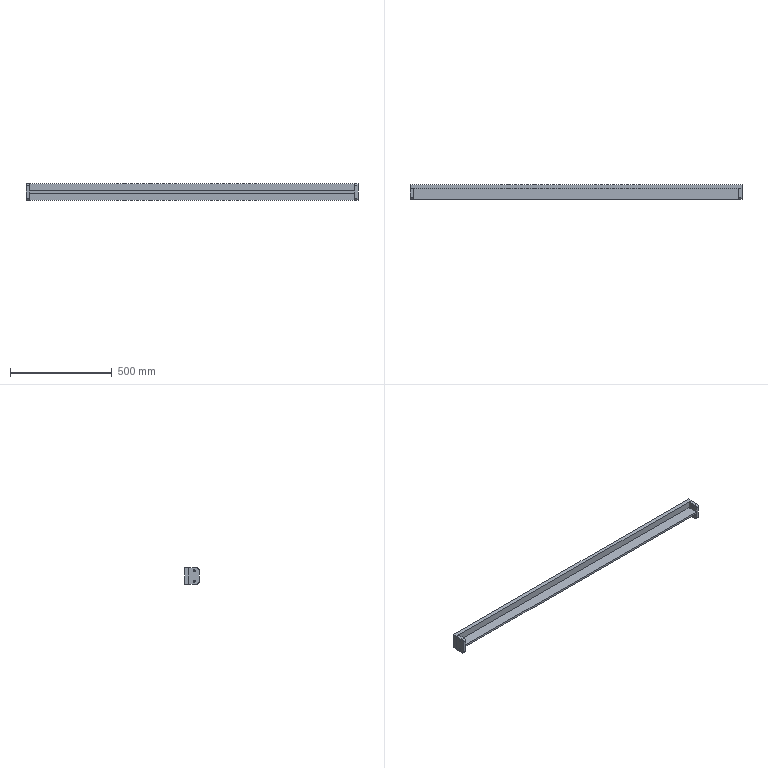Part | SolidWorks | features BaseBody 4 | 4 solids | 36 faces | box 1632 x 70 x 80 mm | volume 3525010 mm3 | plane 24 | cylinder 12 | commonest cylinder face diameters 10.2 x8 20 x4
STEP:
#1=CARTESIAN_POINT('',(-816.,-10.,-40.));
#2=VERTEX_POINT('',#1);
#3=CARTESIAN_POINT('',(-816.,10.,-40.));
#4=VERTEX_POINT('',#3);
#5=CARTESIAN_POINT('',(-816.,10.,-40.));
#6=DIRECTION('',(0.,1.,0.));
#7=VECTOR('',#6,1000.);
#8=LINE('',#5,#7);
#9=EDGE_CURVE('',#2,#4,#8,.T.);
#10=ORIENTED_EDGE('',*,*,#9,.T.);
#11=CARTESIAN_POINT('',(816.,10.,-40.));
#12=VERTEX_POINT('',#11);
#13=CARTESIAN_POINT('',(816.,10.,-40.));
#14=DIRECTION('',(-1.,0.,0.));
#15=VECTOR('',#14,1000.);
#16=LINE('',#13,#15);
#17=EDGE_CURVE('',#12,#4,#16,.T.);
#18=ORIENTED_EDGE('',*,*,#17,.F.);
#19=CARTESIAN_POINT('',(816.,-10.,-40.));
#20=VERTEX_POINT('',#19);
#21=CARTESIAN_POINT('',(816.,10.,-40.));
#22=DIRECTION('',(0.,1.,0.));
#23=VECTOR('',#22,1000.);
#24=LINE('',#21,#23);
#25=EDGE_CURVE('',#20,#12,#24,.T.);
#26=ORIENTED_EDGE('',*,*,#25,.F.);
#27=CARTESIAN_POINT('',(816.,-10.,-40.));
#28=DIRECTION('',(-1.,0.,0.));
#29=VECTOR('',#28,1000.);
#30=LINE('',#27,#29);
#31=EDGE_CURVE('',#20,#2,#30,.T.);
#32=ORIENTED_EDGE('',*,*,#31,.T.);
#33=EDGE_LOOP('',(#10,#18,#26,#32));
#34=FACE_OUTER_BOUND('',#33,.T.);
#35=CARTESIAN_POINT('',(816.,10.,-40.));
#36=DIRECTION('',(0.,0.,1.));
#37=DIRECTION('',(1.,0.,0.));
#38=AXIS2_PLACEMENT_3D('',#35,#36,#37);
#39=PLANE('',#38);
#40=ADVANCED_FACE('',(#34),#39,.F.);
#41=CARTESIAN_POINT('',(-816.,10.,40.));
#42=VERTEX_POINT('',#41);
#43=CARTESIAN_POINT('',(-816.,10.,40.));
#44=DIRECTION('',(0.,0.,1.));
#45=VECTOR('',#44,1000.);
#46=LINE('',#43,#45);
#47=EDGE_CURVE('',#4,#42,#46,.T.);
#48=ORIENTED_EDGE('',*,*,#47,.T.);
#49=CARTESIAN_POINT('',(816.,10.,40.));
#50=VERTEX_POINT('',#49);
#51=CARTESIAN_POINT('',(816.,10.,40.));
#52=DIRECTION('',(-1.,0.,0.));
#53=VECTOR('',#52,1000.);
#54=LINE('',#51,#53);
#55=EDGE_CURVE('',#50,#42,#54,.T.);
#56=ORIENTED_EDGE('',*,*,#55,.F.);
#57=CARTESIAN_POINT('',(816.,10.,40.));
#58=DIRECTION('',(0.,0.,1.));
#59=VECTOR('',#58,1000.);
#60=LINE('',#57,#59);
#61=EDGE_CURVE('',#12,#50,#60,.T.);
#62=ORIENTED_EDGE('',*,*,#61,.F.);
#63=ORIENTED_EDGE('',*,*,#17,.T.);
#64=EDGE_LOOP('',(#48,#56,#62,#63));
#65=FACE_OUTER_BOUND('',#64,.T.);
#66=CARTESIAN_POINT('',(816.,10.,40.));
#67=DIRECTION('',(0.,-1.,0.));
#68=DIRECTION('',(0.,0.,-1.));
#69=AXIS2_PLACEMENT_3D('',#66,#67,#68);
#70=PLANE('',#69);
#71=ADVANCED_FACE('',(#65),#70,.F.);
#72=CARTESIAN_POINT('',(-816.,-10.,40.));
#73=VERTEX_POINT('',#72);
#74=CARTESIAN_POINT('',(-816.,10.,40.));
#75=DIRECTION('',(0.,-1.,0.));
#76=VECTOR('',#75,1000.);
#77=LINE('',#74,#76);
#78=EDGE_CURVE('',#42,#73,#77,.T.);
#79=ORIENTED_EDGE('',*,*,#78,.T.);
#80=CARTESIAN_POINT('',(816.,-10.,40.));
#81=VERTEX_POINT('',#80);
#82=CARTESIAN_POINT('',(816.,-10.,40.));
#83=DIRECTION('',(-1.,0.,0.));
#84=VECTOR('',#83,1000.);
#85=LINE('',#82,#84);
#86=EDGE_CURVE('',#81,#73,#85,.T.);
#87=ORIENTED_EDGE('',*,*,#86,.F.);
#88=CARTESIAN_POINT('',(816.,10.,40.));
#89=DIRECTION('',(0.,-1.,0.));
#90=VECTOR('',#89,1000.);
#91=LINE('',#88,#90);
#92=EDGE_CURVE('',#50,#81,#91,.T.);
#93=ORIENTED_EDGE('',*,*,#92,.F.);
#94=ORIENTED_EDGE('',*,*,#55,.T.);
#95=EDGE_LOOP('',(#79,#87,#93,#94));
#96=FACE_OUTER_BOUND('',#95,.T.);
#97=CARTESIAN_POINT('',(816.,10.,40.));
#98=DIRECTION('',(0.,0.,-1.));
#99=DIRECTION('',(-1.,0.,0.));
#100=AXIS2_PLACEMENT_3D('',#97,#98,#99);
#101=PLANE('',#100);
#102=ADVANCED_FACE('',(#96),#101,.F.);
#103=CARTESIAN_POINT('',(-816.,-10.,40.));
#104=DIRECTION('',(0.,0.,-1.));
#105=VECTOR('',#104,1000.);
#106=LINE('',#103,#105);
#107=EDGE_CURVE('',#73,#2,#106,.T.);
#108=ORIENTED_EDGE('',*,*,#107,.T.);
#109=ORIENTED_EDGE('',*,*,#31,.F.);
#110=CARTESIAN_POINT('',(816.,-10.,40.));
#111=DIRECTION('',(0.,0.,-1.));
#112=VECTOR('',#111,1000.);
#113=LINE('',#110,#112);
#114=EDGE_CURVE('',#81,#20,#113,.T.);
#115=ORIENTED_EDGE('',*,*,#114,.F.);
#116=ORIENTED_EDGE('',*,*,#86,.T.);
#117=EDGE_LOOP('',(#108,#109,#115,#116));
#118=FACE_OUTER_BOUND('',#117,.T.);
#119=CARTESIAN_POINT('',(816.,-10.,40.));
#120=DIRECTION('',(0.,1.,0.));
#121=DIRECTION('',(0.,0.,1.));
#122=AXIS2_PLACEMENT_3D('',#119,#120,#121);
#123=PLANE('',#122);
#124=ADVANCED_FACE('',(#118),#123,.F.);
#125=ORIENTED_EDGE('',*,*,#25,.T.);
#126=ORIENTED_EDGE('',*,*,#61,.T.);
#127=ORIENTED_EDGE('',*,*,#92,.T.);
#128=ORIENTED_EDGE('',*,*,#114,.T.);
#129=EDGE_LOOP('',(#125,#126,#127,#128));
#130=FACE_OUTER_BOUND('',#129,.T.);
#131=CARTESIAN_POINT('',(816.,0.,0.));
#132=DIRECTION('',(1.,0.,0.));
#133=DIRECTION('',(0.,0.,-1.));
#134=AXIS2_PLACEMENT_3D('',#131,#132,#133);
#135=PLANE('',#134);
#136=ADVANCED_FACE('',(#130),#135,.T.);
#137=ORIENTED_EDGE('',*,*,#9,.F.);
#138=ORIENTED_EDGE('',*,*,#107,.F.);
#139=ORIENTED_EDGE('',*,*,#78,.F.);
#140=ORIENTED_EDGE('',*,*,#47,.F.);
#141=EDGE_LOOP('',(#137,#138,#139,#140));
#142=FACE_OUTER_BOUND('',#141,.T.);
#143=CARTESIAN_POINT('',(-816.,0.,0.));
#144=DIRECTION('',(1.,0.,0.));
#145=DIRECTION('',(0.,0.,-1.));
#146=AXIS2_PLACEMENT_3D('',#143,#144,#145);
#147=PLANE('',#146);
#148=ADVANCED_FACE('',(#142),#147,.F.);
#149=CLOSED_SHELL('',(#40,#71,#102,#124,#136,#148));
#150=MANIFOLD_SOLID_BREP('',#149);
#151=CARTESIAN_POINT('',(-800.,-10.,5.));
#152=VERTEX_POINT('',#151);
#153=CARTESIAN_POINT('',(-800.,-60.,5.));
#154=VERTEX_POINT('',#153);
#155=CARTESIAN_POINT('',(-800.,-10.,5.));
#156=DIRECTION('',(0.,-1.,0.));
#157=VECTOR('',#156,1000.);
#158=LINE('',#155,#157);
#159=EDGE_CURVE('',#152,#154,#158,.T.);
#160=ORIENTED_EDGE('',*,*,#159,.T.);
#161=CARTESIAN_POINT('',(800.,-60.,5.));
#162=VERTEX_POINT('',#161);
#163=CARTESIAN_POINT('',(800.,-60.,5.));
#164=DIRECTION('',(-1.,0.,0.));
#165=VECTOR('',#164,1000.);
#166=LINE('',#163,#165);
#167=EDGE_CURVE('',#162,#154,#166,.T.);
#168=ORIENTED_EDGE('',*,*,#167,.F.);
#169=CARTESIAN_POINT('',(800.,-10.,5.));
#170=VERTEX_POINT('',#169);
#171=CARTESIAN_POINT('',(800.,-10.,5.));
#172=DIRECTION('',(0.,-1.,0.));
#173=VECTOR('',#172,1000.);
#174=LINE('',#171,#173);
#175=EDGE_CURVE('',#170,#162,#174,.T.);
#176=ORIENTED_EDGE('',*,*,#175,.F.);
#177=CARTESIAN_POINT('',(800.,-10.,5.));
#178=DIRECTION('',(-1.,0.,0.));
#179=VECTOR('',#178,1000.);
#180=LINE('',#177,#179);
#181=EDGE_CURVE('',#170,#152,#180,.T.);
#182=ORIENTED_EDGE('',*,*,#181,.T.);
#183=EDGE_LOOP('',(#160,#168,#176,#182));
#184=FACE_OUTER_BOUND('',#183,.T.);
#185=CARTESIAN_POINT('',(800.,-10.,5.));
#186=DIRECTION('',(0.,0.,-1.));
#187=DIRECTION('',(0.,1.,0.));
#188=AXIS2_PLACEMENT_3D('',#185,#186,#187);
#189=PLANE('',#188);
#190=ADVANCED_FACE('',(#184),#189,.F.);
#191=CARTESIAN_POINT('',(-800.,-60.,-5.));
#192=VERTEX_POINT('',#191);
#193=CARTESIAN_POINT('',(-800.,-60.,5.));
#194=DIRECTION('',(0.,0.,-1.));
#195=VECTOR('',#194,1000.);
#196=LINE('',#193,#195);
#197=EDGE_CURVE('',#154,#192,#196,.T.);
#198=ORIENTED_EDGE('',*,*,#197,.T.);
#199=CARTESIAN_POINT('',(800.,-60.,-5.));
#200=VERTEX_POINT('',#199);
#201=CARTESIAN_POINT('',(800.,-60.,-5.));
#202=DIRECTION('',(-1.,0.,0.));
#203=VECTOR('',#202,1000.);
#204=LINE('',#201,#203);
#205=EDGE_CURVE('',#200,#192,#204,.T.);
#206=ORIENTED_EDGE('',*,*,#205,.F.);
#207=CARTESIAN_POINT('',(800.,-60.,5.));
#208=DIRECTION('',(0.,0.,-1.));
#209=VECTOR('',#208,1000.);
#210=LINE('',#207,#209);
#211=EDGE_CURVE('',#162,#200,#210,.T.);
#212=ORIENTED_EDGE('',*,*,#211,.F.);
#213=ORIENTED_EDGE('',*,*,#167,.T.);
#214=EDGE_LOOP('',(#198,#206,#212,#213));
#215=FACE_OUTER_BOUND('',#214,.T.);
#216=CARTESIAN_POINT('',(800.,-60.,5.));
#217=DIRECTION('',(0.,1.,0.));
#218=DIRECTION('',(0.,0.,1.));
#219=AXIS2_PLACEMENT_3D('',#216,#217,#218);
#220=PLANE('',#219);
#221=ADVANCED_FACE('',(#215),#220,.F.);
#222=CARTESIAN_POINT('',(-800.,-10.,-5.));
#223=VERTEX_POINT('',#222);
#224=CARTESIAN_POINT('',(-800.,-10.,-5.));
#225=DIRECTION('',(0.,1.,0.));
#226=VECTOR('',#225,1000.);
#227=LINE('',#224,#226);
#228=EDGE_CURVE('',#192,#223,#227,.T.);
#229=ORIENTED_EDGE('',*,*,#228,.T.);
#230=CARTESIAN_POINT('',(800.,-10.,-5.));
#231=VERTEX_POINT('',#230);
#232=CARTESIAN_POINT('',(800.,-10.,-5.));
#233=DIRECTION('',(-1.,0.,0.));
#234=VECTOR('',#233,1000.);
#235=LINE('',#232,#234);
#236=EDGE_CURVE('',#231,#223,#235,.T.);
#237=ORIENTED_EDGE('',*,*,#236,.F.);
#238=CARTESIAN_POINT('',(800.,-10.,-5.));
#239=DIRECTION('',(0.,1.,0.));
#240=VECTOR('',#239,1000.);
#241=LINE('',#238,#240);
#242=EDGE_CURVE('',#200,#231,#241,.T.);
#243=ORIENTED_EDGE('',*,*,#242,.F.);
#244=ORIENTED_EDGE('',*,*,#205,.T.);
#245=EDGE_LOOP('',(#229,#237,#243,#244));
#246=FACE_OUTER_BOUND('',#245,.T.);
#247=CARTESIAN_POINT('',(800.,-10.,-5.));
#248=DIRECTION('',(0.,0.,1.));
#249=DIRECTION('',(0.,-1.,0.));
#250=AXIS2_PLACEMENT_3D('',#247,#248,#249);
#251=PLANE('',#250);
#252=ADVANCED_FACE('',(#246),#251,.F.);
#253=CARTESIAN_POINT('',(-800.,-10.,5.));
#254=DIRECTION('',(0.,0.,1.));
#255=VECTOR('',#254,1000.);
#256=LINE('',#253,#255);
#257=EDGE_CURVE('',#223,#152,#256,.T.);
#258=ORIENTED_EDGE('',*,*,#257,.T.);
#259=ORIENTED_EDGE('',*,*,#181,.F.);
#260=CARTESIAN_POINT('',(800.,-10.,5.));
#261=DIRECTION('',(0.,0.,1.));
#262=VECTOR('',#261,1000.);
#263=LINE('',#260,#262);
#264=EDGE_CURVE('',#231,#170,#263,.T.);
#265=ORIENTED_EDGE('',*,*,#264,.F.);
#266=ORIENTED_EDGE('',*,*,#236,.T.);
#267=EDGE_LOOP('',(#258,#259,#265,#266));
#268=FACE_OUTER_BOUND('',#267,.T.);
#269=CARTESIAN_POINT('',(800.,-10.,5.));
#270=DIRECTION('',(0.,-1.,0.));
#271=DIRECTION('',(0.,0.,-1.));
#272=AXIS2_PLACEMENT_3D('',#269,#270,#271);
#273=PLANE('',#272);
#274=ADVANCED_FACE('',(#268),#273,.F.);
#275=ORIENTED_EDGE('',*,*,#175,.T.);
#276=ORIENTED_EDGE('',*,*,#211,.T.);
#277=ORIENTED_EDGE('',*,*,#242,.T.);
#278=ORIENTED_EDGE('',*,*,#264,.T.);
#279=EDGE_LOOP('',(#275,#276,#277,#278));
#280=FACE_OUTER_BOUND('',#279,.T.);
#281=CARTESIAN_POINT('',(800.,0.,0.));
#282=DIRECTION('',(1.,0.,0.));
#283=DIRECTION('',(0.,0.,-1.));
#284=AXIS2_PLACEMENT_3D('',#281,#282,#283);
#285=PLANE('',#284);
#286=ADVANCED_FACE('',(#280),#285,.T.);
#287=ORIENTED_EDGE('',*,*,#159,.F.);
#288=ORIENTED_EDGE('',*,*,#257,.F.);
#289=ORIENTED_EDGE('',*,*,#228,.F.);
#290=ORIENTED_EDGE('',*,*,#197,.F.);
#291=EDGE_LOOP('',(#287,#288,#289,#290));
#292=FACE_OUTER_BOUND('',#291,.T.);
#293=CARTESIAN_POINT('',(-800.,0.,0.));
#294=DIRECTION('',(1.,0.,0.));
#295=DIRECTION('',(0.,0.,-1.));
#296=AXIS2_PLACEMENT_3D('',#293,#294,#295);
#297=PLANE('',#296);
#298=ADVANCED_FACE('',(#292),#297,.F.);
#299=CLOSED_SHELL('',(#190,#221,#252,#274,#286,#298));
#300=MANIFOLD_SOLID_BREP('',#299);
#301=CARTESIAN_POINT('',(-801.,-35.,19.9));
#302=VERTEX_POINT('',#301);
#303=CARTESIAN_POINT('',(-801.,-35.,30.1));
#304=VERTEX_POINT('',#303);
#305=CARTESIAN_POINT('',(-801.,-35.,25.));
#306=DIRECTION('',(-1.,0.,0.));
#307=DIRECTION('',(0.,0.,1.));
#308=AXIS2_PLACEMENT_3D('',#305,#306,#307);
#309=CIRCLE('',#308,5.1);
#310=EDGE_CURVE('',#302,#304,#309,.T.);
#311=ORIENTED_EDGE('',*,*,#310,.F.);
#312=CARTESIAN_POINT('',(-816.,-35.,19.9));
#313=VERTEX_POINT('',#312);
#314=CARTESIAN_POINT('',(-816.,-35.,19.9));
#315=DIRECTION('',(-1.,0.,0.));
#316=VECTOR('',#315,1000.);
#317=LINE('',#314,#316);
#318=EDGE_CURVE('',#302,#313,#317,.T.);
#319=ORIENTED_EDGE('',*,*,#318,.T.);
#320=CARTESIAN_POINT('',(-816.,-35.,30.1));
#321=VERTEX_POINT('',#320);
#322=CARTESIAN_POINT('',(-816.,-35.,25.));
#323=DIRECTION('',(-1.,0.,0.));
#324=DIRECTION('',(0.,0.,1.));
#325=AXIS2_PLACEMENT_3D('',#322,#323,#324);
#326=CIRCLE('',#325,5.1);
#327=EDGE_CURVE('',#313,#321,#326,.T.);
#328=ORIENTED_EDGE('',*,*,#327,.T.);
#329=CARTESIAN_POINT('',(-816.,-35.,30.1));
#330=DIRECTION('',(-1.,0.,0.));
#331=VECTOR('',#330,1000.);
#332=LINE('',#329,#331);
#333=EDGE_CURVE('',#304,#321,#332,.T.);
#334=ORIENTED_EDGE('',*,*,#333,.F.);
#335=EDGE_LOOP('',(#311,#319,#328,#334));
#336=FACE_OUTER_BOUND('',#335,.T.);
#337=CARTESIAN_POINT('',(-816.,-35.,25.));
#338=DIRECTION('',(-1.,0.,0.));
#339=DIRECTION('',(0.,0.,1.));
#340=AXIS2_PLACEMENT_3D('',#337,#338,#339);
#341=CYLINDRICAL_SURFACE('',#340,5.1);
#342=ADVANCED_FACE('',(#336),#341,.F.);
#343=CARTESIAN_POINT('',(-801.,-35.,-30.1));
#344=VERTEX_POINT('',#343);
#345=CARTESIAN_POINT('',(-801.,-35.,-19.9));
#346=VERTEX_POINT('',#345);
#347=CARTESIAN_POINT('',(-801.,-35.,-25.));
#348=DIRECTION('',(-1.,0.,0.));
#349=DIRECTION('',(0.,0.,1.));
#350=AXIS2_PLACEMENT_3D('',#347,#348,#349);
#351=CIRCLE('',#350,5.1);
#352=EDGE_CURVE('',#344,#346,#351,.T.);
#353=ORIENTED_EDGE('',*,*,#352,.F.);
#354=CARTESIAN_POINT('',(-816.,-35.,-30.1));
#355=VERTEX_POINT('',#354);
#356=CARTESIAN_POINT('',(-816.,-35.,-30.1));
#357=DIRECTION('',(-1.,0.,0.));
#358=VECTOR('',#357,1000.);
#359=LINE('',#356,#358);
#360=EDGE_CURVE('',#344,#355,#359,.T.);
#361=ORIENTED_EDGE('',*,*,#360,.T.);
#362=CARTESIAN_POINT('',(-816.,-35.,-19.9));
#363=VERTEX_POINT('',#362);
#364=CARTESIAN_POINT('',(-816.,-35.,-25.));
#365=DIRECTION('',(-1.,0.,0.));
#366=DIRECTION('',(0.,0.,1.));
#367=AXIS2_PLACEMENT_3D('',#364,#365,#366);
#368=CIRCLE('',#367,5.1);
#369=EDGE_CURVE('',#355,#363,#368,.T.);
#370=ORIENTED_EDGE('',*,*,#369,.T.);
#371=CARTESIAN_POINT('',(-816.,-35.,-19.9));
#372=DIRECTION('',(-1.,0.,0.));
#373=VECTOR('',#372,1000.);
#374=LINE('',#371,#373);
#375=EDGE_CURVE('',#346,#363,#374,.T.);
#376=ORIENTED_EDGE('',*,*,#375,.F.);
#377=EDGE_LOOP('',(#353,#361,#370,#376));
#378=FACE_OUTER_BOUND('',#377,.T.);
#379=CARTESIAN_POINT('',(-816.,-35.,-25.));
#380=DIRECTION('',(-1.,0.,0.));
#381=DIRECTION('',(0.,0.,1.));
#382=AXIS2_PLACEMENT_3D('',#379,#380,#381);
#383=CYLINDRICAL_SURFACE('',#382,5.1);
#384=ADVANCED_FACE('',(#378),#383,.F.);
#385=CARTESIAN_POINT('',(-816.,-10.,-40.));
#386=VERTEX_POINT('',#385);
#387=CARTESIAN_POINT('',(-816.,-50.,-40.));
#388=VERTEX_POINT('',#387);
#389=CARTESIAN_POINT('',(-816.,-10.,-40.));
#390=DIRECTION('',(0.,-1.,0.));
#391=VECTOR('',#390,1000.);
#392=LINE('',#389,#391);
#393=EDGE_CURVE('',#386,#388,#392,.T.);
#394=ORIENTED_EDGE('',*,*,#393,.F.);
#395=CARTESIAN_POINT('',(-801.,-10.,-40.));
#396=VERTEX_POINT('',#395);
#397=CARTESIAN_POINT('',(-801.,-10.,-40.));
#398=DIRECTION('',(-1.,0.,0.));
#399=VECTOR('',#398,1000.);
#400=LINE('',#397,#399);
#401=EDGE_CURVE('',#396,#386,#400,.T.);
#402=ORIENTED_EDGE('',*,*,#401,.F.);
#403=CARTESIAN_POINT('',(-801.,-50.,-40.));
#404=VERTEX_POINT('',#403);
#405=CARTESIAN_POINT('',(-801.,-10.,-40.));
#406=DIRECTION('',(0.,-1.,0.));
#407=VECTOR('',#406,1000.);
#408=LINE('',#405,#407);
#409=EDGE_CURVE('',#396,#404,#408,.T.);
#410=ORIENTED_EDGE('',*,*,#409,.T.);
#411=CARTESIAN_POINT('',(-801.,-50.,-40.));
#412=DIRECTION('',(-1.,0.,0.));
#413=VECTOR('',#412,1000.);
#414=LINE('',#411,#413);
#415=EDGE_CURVE('',#404,#388,#414,.T.);
#416=ORIENTED_EDGE('',*,*,#415,.T.);
#417=EDGE_LOOP('',(#394,#402,#410,#416));
#418=FACE_OUTER_BOUND('',#417,.T.);
#419=CARTESIAN_POINT('',(-801.,-10.,-40.));
#420=DIRECTION('',(0.,0.,-1.));
#421=DIRECTION('',(0.,1.,0.));
#422=AXIS2_PLACEMENT_3D('',#419,#420,#421);
#423=PLANE('',#422);
#424=ADVANCED_FACE('',(#418),#423,.T.);
#425=CARTESIAN_POINT('',(-816.,-10.,40.));
#426=VERTEX_POINT('',#425);
#427=CARTESIAN_POINT('',(-816.,-10.,-40.));
#428=DIRECTION('',(0.,0.,-1.));
#429=VECTOR('',#428,1000.);
#430=LINE('',#427,#429);
#431=EDGE_CURVE('',#426,#386,#430,.T.);
#432=ORIENTED_EDGE('',*,*,#431,.F.);
#433=CARTESIAN_POINT('',(-801.,-10.,40.));
#434=VERTEX_POINT('',#433);
#435=CARTESIAN_POINT('',(-801.,-10.,40.));
#436=DIRECTION('',(-1.,0.,0.));
#437=VECTOR('',#436,1000.);
#438=LINE('',#435,#437);
#439=EDGE_CURVE('',#434,#426,#438,.T.);
#440=ORIENTED_EDGE('',*,*,#439,.F.);
#441=CARTESIAN_POINT('',(-801.,-10.,-40.));
#442=DIRECTION('',(0.,0.,-1.));
#443=VECTOR('',#442,1000.);
#444=LINE('',#441,#443);
#445=EDGE_CURVE('',#434,#396,#444,.T.);
#446=ORIENTED_EDGE('',*,*,#445,.T.);
#447=ORIENTED_EDGE('',*,*,#401,.T.);
#448=EDGE_LOOP('',(#432,#440,#446,#447));
#449=FACE_OUTER_BOUND('',#448,.T.);
#450=CARTESIAN_POINT('',(-801.,-10.,-40.));
#451=DIRECTION('',(0.,1.,0.));
#452=DIRECTION('',(0.,0.,1.));
#453=AXIS2_PLACEMENT_3D('',#450,#451,#452);
#454=PLANE('',#453);
#455=ADVANCED_FACE('',(#449),#454,.T.);
#456=CARTESIAN_POINT('',(-816.,-50.,40.));
#457=VERTEX_POINT('',#456);
#458=CARTESIAN_POINT('',(-816.,-10.,40.));
#459=DIRECTION('',(0.,1.,0.));
#460=VECTOR('',#459,1000.);
#461=LINE('',#458,#460);
#462=EDGE_CURVE('',#457,#426,#461,.T.);
#463=ORIENTED_EDGE('',*,*,#462,.F.);
#464=CARTESIAN_POINT('',(-801.,-50.,40.));
#465=VERTEX_POINT('',#464);
#466=CARTESIAN_POINT('',(-801.,-50.,40.));
#467=DIRECTION('',(-1.,0.,0.));
#468=VECTOR('',#467,1000.);
#469=LINE('',#466,#468);
#470=EDGE_CURVE('',#465,#457,#469,.T.);
#471=ORIENTED_EDGE('',*,*,#470,.F.);
#472=CARTESIAN_POINT('',(-801.,-10.,40.));
#473=DIRECTION('',(0.,1.,0.));
#474=VECTOR('',#473,1000.);
#475=LINE('',#472,#474);
#476=EDGE_CURVE('',#465,#434,#475,.T.);
#477=ORIENTED_EDGE('',*,*,#476,.T.);
#478=ORIENTED_EDGE('',*,*,#439,.T.);
#479=EDGE_LOOP('',(#463,#471,#477,#478));
#480=FACE_OUTER_BOUND('',#479,.T.);
#481=CARTESIAN_POINT('',(-801.,-10.,40.));
#482=DIRECTION('',(0.,0.,1.));
#483=DIRECTION('',(1.,0.,0.));
#484=AXIS2_PLACEMENT_3D('',#481,#482,#483);
#485=PLANE('',#484);
#486=ADVANCED_FACE('',(#480),#485,.T.);
#487=CARTESIAN_POINT('',(-816.,-60.,30.));
#488=VERTEX_POINT('',#487);
#489=CARTESIAN_POINT('',(-816.,-50.,30.));
#490=DIRECTION('',(-1.,0.,0.));
#491=DIRECTION('',(0.,0.,1.));
#492=AXIS2_PLACEMENT_3D('',#489,#490,#491);
#493=CIRCLE('',#492,10.);
#494=EDGE_CURVE('',#488,#457,#493,.T.);
#495=ORIENTED_EDGE('',*,*,#494,.F.);
#496=CARTESIAN_POINT('',(-801.,-60.,30.));
#497=VERTEX_POINT('',#496);
#498=CARTESIAN_POINT('',(-801.,-60.,30.));
#499=DIRECTION('',(-1.,0.,0.));
#500=VECTOR('',#499,1000.);
#501=LINE('',#498,#500);
#502=EDGE_CURVE('',#497,#488,#501,.T.);
#503=ORIENTED_EDGE('',*,*,#502,.F.);
#504=CARTESIAN_POINT('',(-801.,-50.,30.));
#505=DIRECTION('',(-1.,0.,0.));
#506=DIRECTION('',(0.,0.,1.));
#507=AXIS2_PLACEMENT_3D('',#504,#505,#506);
#508=CIRCLE('',#507,10.);
#509=EDGE_CURVE('',#497,#465,#508,.T.);
#510=ORIENTED_EDGE('',*,*,#509,.T.);
#511=ORIENTED_EDGE('',*,*,#470,.T.);
#512=EDGE_LOOP('',(#495,#503,#510,#511));
#513=FACE_OUTER_BOUND('',#512,.T.);
#514=CARTESIAN_POINT('',(-801.,-50.,30.));
#515=DIRECTION('',(-1.,0.,0.));
#516=DIRECTION('',(0.,0.,1.));
#517=AXIS2_PLACEMENT_3D('',#514,#515,#516);
#518=CYLINDRICAL_SURFACE('',#517,10.);
#519=ADVANCED_FACE('',(#513),#518,.T.);
#520=CARTESIAN_POINT('',(-816.,-60.,-30.));
#521=VERTEX_POINT('',#520);
#522=CARTESIAN_POINT('',(-816.,-60.,-30.));
#523=DIRECTION('',(0.,0.,1.));
#524=VECTOR('',#523,1000.);
#525=LINE('',#522,#524);
#526=EDGE_CURVE('',#521,#488,#525,.T.);
#527=ORIENTED_EDGE('',*,*,#526,.F.);
#528=CARTESIAN_POINT('',(-801.,-60.,-30.));
#529=VERTEX_POINT('',#528);
#530=CARTESIAN_POINT('',(-801.,-60.,-30.));
#531=DIRECTION('',(-1.,0.,0.));
#532=VECTOR('',#531,1000.);
#533=LINE('',#530,#532);
#534=EDGE_CURVE('',#529,#521,#533,.T.);
#535=ORIENTED_EDGE('',*,*,#534,.F.);
#536=CARTESIAN_POINT('',(-801.,-60.,-30.));
#537=DIRECTION('',(0.,0.,1.));
#538=VECTOR('',#537,1000.);
#539=LINE('',#536,#538);
#540=EDGE_CURVE('',#529,#497,#539,.T.);
#541=ORIENTED_EDGE('',*,*,#540,.T.);
#542=ORIENTED_EDGE('',*,*,#502,.T.);
#543=EDGE_LOOP('',(#527,#535,#541,#542));
#544=FACE_OUTER_BOUND('',#543,.T.);
#545=CARTESIAN_POINT('',(-801.,-60.,-30.));
#546=DIRECTION('',(0.,-1.,0.));
#547=DIRECTION('',(0.,0.,-1.));
#548=AXIS2_PLACEMENT_3D('',#545,#546,#547);
#549=PLANE('',#548);
#550=ADVANCED_FACE('',(#544),#549,.T.);
#551=CARTESIAN_POINT('',(-816.,-50.,-30.));
#552=DIRECTION('',(-1.,0.,0.));
#553=DIRECTION('',(0.,0.,1.));
#554=AXIS2_PLACEMENT_3D('',#551,#552,#553);
#555=CIRCLE('',#554,10.);
#556=EDGE_CURVE('',#388,#521,#555,.T.);
#557=ORIENTED_EDGE('',*,*,#556,.F.);
#558=ORIENTED_EDGE('',*,*,#415,.F.);
#559=CARTESIAN_POINT('',(-801.,-50.,-30.));
#560=DIRECTION('',(-1.,0.,0.));
#561=DIRECTION('',(0.,0.,1.));
#562=AXIS2_PLACEMENT_3D('',#559,#560,#561);
#563=CIRCLE('',#562,10.);
#564=EDGE_CURVE('',#404,#529,#563,.T.);
#565=ORIENTED_EDGE('',*,*,#564,.T.);
#566=ORIENTED_EDGE('',*,*,#534,.T.);
#567=EDGE_LOOP('',(#557,#558,#565,#566));
#568=FACE_OUTER_BOUND('',#567,.T.);
#569=CARTESIAN_POINT('',(-801.,-50.,-30.));
#570=DIRECTION('',(-1.,0.,0.));
#571=DIRECTION('',(0.,0.,1.));
#572=AXIS2_PLACEMENT_3D('',#569,#570,#571);
#573=CYLINDRICAL_SURFACE('',#572,10.);
#574=ADVANCED_FACE('',(#568),#573,.T.);
#575=CARTESIAN_POINT('',(-801.,-35.,25.));
#576=DIRECTION('',(-1.,0.,0.));
#577=DIRECTION('',(0.,0.,1.));
#578=AXIS2_PLACEMENT_3D('',#575,#576,#577);
#579=CIRCLE('',#578,5.1);
#580=EDGE_CURVE('',#304,#302,#579,.T.);
#581=ORIENTED_EDGE('',*,*,#580,.T.);
#582=ORIENTED_EDGE('',*,*,#310,.T.);
#583=EDGE_LOOP('',(#581,#582));
#584=FACE_BOUND('',#583,.T.);
#585=CARTESIAN_POINT('',(-801.,-35.,-25.));
#586=DIRECTION('',(-1.,0.,0.));
#587=DIRECTION('',(0.,0.,1.));
#588=AXIS2_PLACEMENT_3D('',#585,#586,#587);
#589=CIRCLE('',#588,5.1);
#590=EDGE_CURVE('',#346,#344,#589,.T.);
#591=ORIENTED_EDGE('',*,*,#590,.T.);
#592=ORIENTED_EDGE('',*,*,#352,.T.);
#593=EDGE_LOOP('',(#591,#592));
#594=FACE_BOUND('',#593,.T.);
#595=ORIENTED_EDGE('',*,*,#409,.F.);
#596=ORIENTED_EDGE('',*,*,#445,.F.);
#597=ORIENTED_EDGE('',*,*,#476,.F.);
#598=ORIENTED_EDGE('',*,*,#509,.F.);
#599=ORIENTED_EDGE('',*,*,#540,.F.);
#600=ORIENTED_EDGE('',*,*,#564,.F.);
#601=EDGE_LOOP('',(#595,#596,#597,#598,#599,#600));
#602=FACE_OUTER_BOUND('',#601,.T.);
#603=CARTESIAN_POINT('',(-801.,-50.,-30.));
#604=DIRECTION('',(-1.,0.,0.));
#605=DIRECTION('',(0.,0.,1.));
#606=AXIS2_PLACEMENT_3D('',#603,#604,#605);
#607=PLANE('',#606);
#608=ADVANCED_FACE('',(#584,#594,#602),#607,.F.);
#609=CARTESIAN_POINT('',(-816.,-35.,25.));
#610=DIRECTION('',(-1.,0.,0.));
#611=DIRECTION('',(0.,0.,1.));
#612=AXIS2_PLACEMENT_3D('',#609,#610,#611);
#613=CIRCLE('',#612,5.1);
#614=EDGE_CURVE('',#321,#313,#613,.T.);
#615=ORIENTED_EDGE('',*,*,#614,.F.);
#616=ORIENTED_EDGE('',*,*,#327,.F.);
#617=EDGE_LOOP('',(#615,#616));
#618=FACE_BOUND('',#617,.T.);
#619=CARTESIAN_POINT('',(-816.,-35.,-25.));
#620=DIRECTION('',(-1.,0.,0.));
#621=DIRECTION('',(0.,0.,1.));
#622=AXIS2_PLACEMENT_3D('',#619,#620,#621);
#623=CIRCLE('',#622,5.1);
#624=EDGE_CURVE('',#363,#355,#623,.T.);
#625=ORIENTED_EDGE('',*,*,#624,.F.);
#626=ORIENTED_EDGE('',*,*,#369,.F.);
#627=EDGE_LOOP('',(#625,#626));
#628=FACE_BOUND('',#627,.T.);
#629=ORIENTED_EDGE('',*,*,#393,.T.);
#630=ORIENTED_EDGE('',*,*,#556,.T.);
#631=ORIENTED_EDGE('',*,*,#526,.T.);
#632=ORIENTED_EDGE('',*,*,#494,.T.);
#633=ORIENTED_EDGE('',*,*,#462,.T.);
#634=ORIENTED_EDGE('',*,*,#431,.T.);
#635=EDGE_LOOP('',(#629,#630,#631,#632,#633,#634));
#636=FACE_OUTER_BOUND('',#635,.T.);
#637=CARTESIAN_POINT('',(-816.,-50.,-30.));
#638=DIRECTION('',(-1.,0.,0.));
#639=DIRECTION('',(0.,0.,1.));
#640=AXIS2_PLACEMENT_3D('',#637,#638,#639);
#641=PLANE('',#640);
#642=ADVANCED_FACE('',(#618,#628,#636),#641,.T.);
#643=ORIENTED_EDGE('',*,*,#360,.F.);
#644=ORIENTED_EDGE('',*,*,#590,.F.);
#645=ORIENTED_EDGE('',*,*,#375,.T.);
#646=ORIENTED_EDGE('',*,*,#624,.T.);
#647=EDGE_LOOP('',(#643,#644,#645,#646));
#648=FACE_OUTER_BOUND('',#647,.T.);
#649=CARTESIAN_POINT('',(-816.,-35.,-25.));
#650=DIRECTION('',(-1.,0.,0.));
#651=DIRECTION('',(0.,0.,1.));
#652=AXIS2_PLACEMENT_3D('',#649,#650,#651);
#653=CYLINDRICAL_SURFACE('',#652,5.1);
#654=ADVANCED_FACE('',(#648),#653,.F.);
#655=ORIENTED_EDGE('',*,*,#318,.F.);
#656=ORIENTED_EDGE('',*,*,#580,.F.);
#657=ORIENTED_EDGE('',*,*,#333,.T.);
#658=ORIENTED_EDGE('',*,*,#614,.T.);
#659=EDGE_LOOP('',(#655,#656,#657,#658));
#660=FACE_OUTER_BOUND('',#659,.T.);
#661=CARTESIAN_POINT('',(-816.,-35.,25.));
#662=DIRECTION('',(-1.,0.,0.));
#663=DIRECTION('',(0.,0.,1.));
#664=AXIS2_PLACEMENT_3D('',#661,#662,#663);
#665=CYLINDRICAL_SURFACE('',#664,5.1);
#666=ADVANCED_FACE('',(#660),#665,.F.);
#667=CLOSED_SHELL('',(#342,#384,#424,#455,#486,#519,#550,#574,#608,#642,#654,#666));
#668=MANIFOLD_SOLID_BREP('',#667);
#669=CARTESIAN_POINT('',(801.,-35.,30.1));
#670=VERTEX_POINT('',#669);
#671=CARTESIAN_POINT('',(801.,-35.,19.9));
#672=VERTEX_POINT('',#671);
#673=CARTESIAN_POINT('',(801.,-35.,25.));
#674=DIRECTION('',(-1.,0.,0.));
#675=DIRECTION('',(0.,0.,1.));
#676=AXIS2_PLACEMENT_3D('',#673,#674,#675);
#677=CIRCLE('',#676,5.1);
#678=EDGE_CURVE('',#670,#672,#677,.T.);
#679=ORIENTED_EDGE('',*,*,#678,.T.);
#680=CARTESIAN_POINT('',(816.,-35.,19.9));
#681=VERTEX_POINT('',#680);
#682=CARTESIAN_POINT('',(816.,-35.,19.9));
#683=DIRECTION('',(1.,0.,0.));
#684=VECTOR('',#683,1000.);
#685=LINE('',#682,#684);
#686=EDGE_CURVE('',#672,#681,#685,.T.);
#687=ORIENTED_EDGE('',*,*,#686,.T.);
#688=CARTESIAN_POINT('',(816.,-35.,30.1));
#689=VERTEX_POINT('',#688);
#690=CARTESIAN_POINT('',(816.,-35.,25.));
#691=DIRECTION('',(-1.,0.,0.));
#692=DIRECTION('',(0.,0.,1.));
#693=AXIS2_PLACEMENT_3D('',#690,#691,#692);
#694=CIRCLE('',#693,5.1);
#695=EDGE_CURVE('',#689,#681,#694,.T.);
#696=ORIENTED_EDGE('',*,*,#695,.F.);
#697=CARTESIAN_POINT('',(816.,-35.,30.1));
#698=DIRECTION('',(1.,0.,0.));
#699=VECTOR('',#698,1000.);
#700=LINE('',#697,#699);
#701=EDGE_CURVE('',#670,#689,#700,.T.);
#702=ORIENTED_EDGE('',*,*,#701,.F.);
#703=EDGE_LOOP('',(#679,#687,#696,#702));
#704=FACE_OUTER_BOUND('',#703,.T.);
#705=CARTESIAN_POINT('',(816.,-35.,25.));
#706=DIRECTION('',(1.,0.,0.));
#707=DIRECTION('',(0.,0.,1.));
#708=AXIS2_PLACEMENT_3D('',#705,#706,#707);
#709=CYLINDRICAL_SURFACE('',#708,5.1);
#710=ADVANCED_FACE('',(#704),#709,.F.);
#711=CARTESIAN_POINT('',(801.,-35.,-19.9));
#712=VERTEX_POINT('',#711);
#713=CARTESIAN_POINT('',(801.,-35.,-30.1));
#714=VERTEX_POINT('',#713);
#715=CARTESIAN_POINT('',(801.,-35.,-25.));
#716=DIRECTION('',(-1.,0.,0.));
#717=DIRECTION('',(0.,0.,1.));
#718=AXIS2_PLACEMENT_3D('',#715,#716,#717);
#719=CIRCLE('',#718,5.1);
#720=EDGE_CURVE('',#712,#714,#719,.T.);
#721=ORIENTED_EDGE('',*,*,#720,.T.);
#722=CARTESIAN_POINT('',(816.,-35.,-30.1));
#723=VERTEX_POINT('',#722);
#724=CARTESIAN_POINT('',(816.,-35.,-30.1));
#725=DIRECTION('',(1.,0.,0.));
#726=VECTOR('',#725,1000.);
#727=LINE('',#724,#726);
#728=EDGE_CURVE('',#714,#723,#727,.T.);
#729=ORIENTED_EDGE('',*,*,#728,.T.);
#730=CARTESIAN_POINT('',(816.,-35.,-19.9));
#731=VERTEX_POINT('',#730);
#732=CARTESIAN_POINT('',(816.,-35.,-25.));
#733=DIRECTION('',(-1.,0.,0.));
#734=DIRECTION('',(0.,0.,1.));
#735=AXIS2_PLACEMENT_3D('',#732,#733,#734);
#736=CIRCLE('',#735,5.1);
#737=EDGE_CURVE('',#731,#723,#736,.T.);
#738=ORIENTED_EDGE('',*,*,#737,.F.);
#739=CARTESIAN_POINT('',(816.,-35.,-19.9));
#740=DIRECTION('',(1.,0.,0.));
#741=VECTOR('',#740,1000.);
#742=LINE('',#739,#741);
#743=EDGE_CURVE('',#712,#731,#742,.T.);
#744=ORIENTED_EDGE('',*,*,#743,.F.);
#745=EDGE_LOOP('',(#721,#729,#738,#744));
#746=FACE_OUTER_BOUND('',#745,.T.);
#747=CARTESIAN_POINT('',(816.,-35.,-25.));
#748=DIRECTION('',(1.,0.,0.));
#749=DIRECTION('',(0.,0.,1.));
#750=AXIS2_PLACEMENT_3D('',#747,#748,#749);
#751=CYLINDRICAL_SURFACE('',#750,5.1);
#752=ADVANCED_FACE('',(#746),#751,.F.);
#753=CARTESIAN_POINT('',(816.,-10.,-40.));
#754=VERTEX_POINT('',#753);
#755=CARTESIAN_POINT('',(816.,-50.,-40.));
#756=VERTEX_POINT('',#755);
#757=CARTESIAN_POINT('',(816.,-10.,-40.));
#758=DIRECTION('',(0.,-1.,0.));
#759=VECTOR('',#758,1000.);
#760=LINE('',#757,#759);
#761=EDGE_CURVE('',#754,#756,#760,.T.);
#762=ORIENTED_EDGE('',*,*,#761,.T.);
#763=CARTESIAN_POINT('',(801.,-50.,-40.));
#764=VERTEX_POINT('',#763);
#765=CARTESIAN_POINT('',(801.,-50.,-40.));
#766=DIRECTION('',(1.,0.,0.));
#767=VECTOR('',#766,1000.);
#768=LINE('',#765,#767);
#769=EDGE_CURVE('',#764,#756,#768,.T.);
#770=ORIENTED_EDGE('',*,*,#769,.F.);
#771=CARTESIAN_POINT('',(801.,-10.,-40.));
#772=VERTEX_POINT('',#771);
#773=CARTESIAN_POINT('',(801.,-10.,-40.));
#774=DIRECTION('',(0.,-1.,0.));
#775=VECTOR('',#774,1000.);
#776=LINE('',#773,#775);
#777=EDGE_CURVE('',#772,#764,#776,.T.);
#778=ORIENTED_EDGE('',*,*,#777,.F.);
#779=CARTESIAN_POINT('',(801.,-10.,-40.));
#780=DIRECTION('',(1.,0.,0.));
#781=VECTOR('',#780,1000.);
#782=LINE('',#779,#781);
#783=EDGE_CURVE('',#772,#754,#782,.T.);
#784=ORIENTED_EDGE('',*,*,#783,.T.);
#785=EDGE_LOOP('',(#762,#770,#778,#784));
#786=FACE_OUTER_BOUND('',#785,.T.);
#787=CARTESIAN_POINT('',(801.,-10.,-40.));
#788=DIRECTION('',(0.,0.,-1.));
#789=DIRECTION('',(0.,1.,0.));
#790=AXIS2_PLACEMENT_3D('',#787,#788,#789);
#791=PLANE('',#790);
#792=ADVANCED_FACE('',(#786),#791,.T.);
#793=CARTESIAN_POINT('',(816.,-10.,40.));
#794=VERTEX_POINT('',#793);
#795=CARTESIAN_POINT('',(816.,-10.,-40.));
#796=DIRECTION('',(0.,0.,-1.));
#797=VECTOR('',#796,1000.);
#798=LINE('',#795,#797);
#799=EDGE_CURVE('',#794,#754,#798,.T.);
#800=ORIENTED_EDGE('',*,*,#799,.T.);
#801=ORIENTED_EDGE('',*,*,#783,.F.);
#802=CARTESIAN_POINT('',(801.,-10.,40.));
#803=VERTEX_POINT('',#802);
#804=CARTESIAN_POINT('',(801.,-10.,-40.));
#805=DIRECTION('',(0.,0.,-1.));
#806=VECTOR('',#805,1000.);
#807=LINE('',#804,#806);
#808=EDGE_CURVE('',#803,#772,#807,.T.);
#809=ORIENTED_EDGE('',*,*,#808,.F.);
#810=CARTESIAN_POINT('',(801.,-10.,40.));
#811=DIRECTION('',(1.,0.,0.));
#812=VECTOR('',#811,1000.);
#813=LINE('',#810,#812);
#814=EDGE_CURVE('',#803,#794,#813,.T.);
#815=ORIENTED_EDGE('',*,*,#814,.T.);
#816=EDGE_LOOP('',(#800,#801,#809,#815));
#817=FACE_OUTER_BOUND('',#816,.T.);
#818=CARTESIAN_POINT('',(801.,-10.,-40.));
#819=DIRECTION('',(0.,1.,0.));
#820=DIRECTION('',(0.,0.,1.));
#821=AXIS2_PLACEMENT_3D('',#818,#819,#820);
#822=PLANE('',#821);
#823=ADVANCED_FACE('',(#817),#822,.T.);
#824=CARTESIAN_POINT('',(816.,-50.,40.));
#825=VERTEX_POINT('',#824);
#826=CARTESIAN_POINT('',(816.,-10.,40.));
#827=DIRECTION('',(0.,1.,0.));
#828=VECTOR('',#827,1000.);
#829=LINE('',#826,#828);
#830=EDGE_CURVE('',#825,#794,#829,.T.);
#831=ORIENTED_EDGE('',*,*,#830,.T.);
#832=ORIENTED_EDGE('',*,*,#814,.F.);
#833=CARTESIAN_POINT('',(801.,-50.,40.));
#834=VERTEX_POINT('',#833);
#835=CARTESIAN_POINT('',(801.,-10.,40.));
#836=DIRECTION('',(0.,1.,0.));
#837=VECTOR('',#836,1000.);
#838=LINE('',#835,#837);
#839=EDGE_CURVE('',#834,#803,#838,.T.);
#840=ORIENTED_EDGE('',*,*,#839,.F.);
#841=CARTESIAN_POINT('',(801.,-50.,40.));
#842=DIRECTION('',(1.,0.,0.));
#843=VECTOR('',#842,1000.);
#844=LINE('',#841,#843);
#845=EDGE_CURVE('',#834,#825,#844,.T.);
#846=ORIENTED_EDGE('',*,*,#845,.T.);
#847=EDGE_LOOP('',(#831,#832,#840,#846));
#848=FACE_OUTER_BOUND('',#847,.T.);
#849=CARTESIAN_POINT('',(801.,-10.,40.));
#850=DIRECTION('',(0.,0.,1.));
#851=DIRECTION('',(-1.,0.,0.));
#852=AXIS2_PLACEMENT_3D('',#849,#850,#851);
#853=PLANE('',#852);
#854=ADVANCED_FACE('',(#848),#853,.T.);
#855=CARTESIAN_POINT('',(816.,-60.,30.));
#856=VERTEX_POINT('',#855);
#857=CARTESIAN_POINT('',(816.,-50.,30.));
#858=DIRECTION('',(-1.,0.,0.));
#859=DIRECTION('',(0.,0.,1.));
#860=AXIS2_PLACEMENT_3D('',#857,#858,#859);
#861=CIRCLE('',#860,10.);
#862=EDGE_CURVE('',#856,#825,#861,.T.);
#863=ORIENTED_EDGE('',*,*,#862,.T.);
#864=ORIENTED_EDGE('',*,*,#845,.F.);
#865=CARTESIAN_POINT('',(801.,-60.,30.));
#866=VERTEX_POINT('',#865);
#867=CARTESIAN_POINT('',(801.,-50.,30.));
#868=DIRECTION('',(-1.,0.,0.));
#869=DIRECTION('',(0.,0.,1.));
#870=AXIS2_PLACEMENT_3D('',#867,#868,#869);
#871=CIRCLE('',#870,10.);
#872=EDGE_CURVE('',#866,#834,#871,.T.);
#873=ORIENTED_EDGE('',*,*,#872,.F.);
#874=CARTESIAN_POINT('',(801.,-60.,30.));
#875=DIRECTION('',(1.,0.,0.));
#876=VECTOR('',#875,1000.);
#877=LINE('',#874,#876);
#878=EDGE_CURVE('',#866,#856,#877,.T.);
#879=ORIENTED_EDGE('',*,*,#878,.T.);
#880=EDGE_LOOP('',(#863,#864,#873,#879));
#881=FACE_OUTER_BOUND('',#880,.T.);
#882=CARTESIAN_POINT('',(801.,-50.,30.));
#883=DIRECTION('',(1.,0.,0.));
#884=DIRECTION('',(0.,0.,1.));
#885=AXIS2_PLACEMENT_3D('',#882,#883,#884);
#886=CYLINDRICAL_SURFACE('',#885,10.);
#887=ADVANCED_FACE('',(#881),#886,.T.);
#888=CARTESIAN_POINT('',(816.,-60.,-30.));
#889=VERTEX_POINT('',#888);
#890=CARTESIAN_POINT('',(816.,-60.,-30.));
#891=DIRECTION('',(0.,0.,1.));
#892=VECTOR('',#891,1000.);
#893=LINE('',#890,#892);
#894=EDGE_CURVE('',#889,#856,#893,.T.);
#895=ORIENTED_EDGE('',*,*,#894,.T.);
#896=ORIENTED_EDGE('',*,*,#878,.F.);
#897=CARTESIAN_POINT('',(801.,-60.,-30.));
#898=VERTEX_POINT('',#897);
#899=CARTESIAN_POINT('',(801.,-60.,-30.));
#900=DIRECTION('',(0.,0.,1.));
#901=VECTOR('',#900,1000.);
#902=LINE('',#899,#901);
#903=EDGE_CURVE('',#898,#866,#902,.T.);
#904=ORIENTED_EDGE('',*,*,#903,.F.);
#905=CARTESIAN_POINT('',(801.,-60.,-30.));
#906=DIRECTION('',(1.,0.,0.));
#907=VECTOR('',#906,1000.);
#908=LINE('',#905,#907);
#909=EDGE_CURVE('',#898,#889,#908,.T.);
#910=ORIENTED_EDGE('',*,*,#909,.T.);
#911=EDGE_LOOP('',(#895,#896,#904,#910));
#912=FACE_OUTER_BOUND('',#911,.T.);
#913=CARTESIAN_POINT('',(801.,-60.,-30.));
#914=DIRECTION('',(0.,-1.,0.));
#915=DIRECTION('',(0.,0.,-1.));
#916=AXIS2_PLACEMENT_3D('',#913,#914,#915);
#917=PLANE('',#916);
#918=ADVANCED_FACE('',(#912),#917,.T.);
#919=CARTESIAN_POINT('',(816.,-50.,-30.));
#920=DIRECTION('',(-1.,0.,0.));
#921=DIRECTION('',(0.,0.,1.));
#922=AXIS2_PLACEMENT_3D('',#919,#920,#921);
#923=CIRCLE('',#922,10.);
#924=EDGE_CURVE('',#756,#889,#923,.T.);
#925=ORIENTED_EDGE('',*,*,#924,.T.);
#926=ORIENTED_EDGE('',*,*,#909,.F.);
#927=CARTESIAN_POINT('',(801.,-50.,-30.));
#928=DIRECTION('',(-1.,0.,0.));
#929=DIRECTION('',(0.,0.,1.));
#930=AXIS2_PLACEMENT_3D('',#927,#928,#929);
#931=CIRCLE('',#930,10.);
#932=EDGE_CURVE('',#764,#898,#931,.T.);
#933=ORIENTED_EDGE('',*,*,#932,.F.);
#934=ORIENTED_EDGE('',*,*,#769,.T.);
#935=EDGE_LOOP('',(#925,#926,#933,#934));
#936=FACE_OUTER_BOUND('',#935,.T.);
#937=CARTESIAN_POINT('',(801.,-50.,-30.));
#938=DIRECTION('',(1.,0.,0.));
#939=DIRECTION('',(0.,0.,1.));
#940=AXIS2_PLACEMENT_3D('',#937,#938,#939);
#941=CYLINDRICAL_SURFACE('',#940,10.);
#942=ADVANCED_FACE('',(#936),#941,.T.);
#943=ORIENTED_EDGE('',*,*,#678,.F.);
#944=CARTESIAN_POINT('',(801.,-35.,25.));
#945=DIRECTION('',(-1.,0.,0.));
#946=DIRECTION('',(0.,0.,1.));
#947=AXIS2_PLACEMENT_3D('',#944,#945,#946);
#948=CIRCLE('',#947,5.1);
#949=EDGE_CURVE('',#672,#670,#948,.T.);
#950=ORIENTED_EDGE('',*,*,#949,.F.);
#951=EDGE_LOOP('',(#943,#950));
#952=FACE_BOUND('',#951,.T.);
#953=ORIENTED_EDGE('',*,*,#720,.F.);
#954=CARTESIAN_POINT('',(801.,-35.,-25.));
#955=DIRECTION('',(-1.,0.,0.));
#956=DIRECTION('',(0.,0.,1.));
#957=AXIS2_PLACEMENT_3D('',#954,#955,#956);
#958=CIRCLE('',#957,5.1);
#959=EDGE_CURVE('',#714,#712,#958,.T.);
#960=ORIENTED_EDGE('',*,*,#959,.F.);
#961=EDGE_LOOP('',(#953,#960));
#962=FACE_BOUND('',#961,.T.);
#963=ORIENTED_EDGE('',*,*,#777,.T.);
#964=ORIENTED_EDGE('',*,*,#932,.T.);
#965=ORIENTED_EDGE('',*,*,#903,.T.);
#966=ORIENTED_EDGE('',*,*,#872,.T.);
#967=ORIENTED_EDGE('',*,*,#839,.T.);
#968=ORIENTED_EDGE('',*,*,#808,.T.);
#969=EDGE_LOOP('',(#963,#964,#965,#966,#967,#968));
#970=FACE_OUTER_BOUND('',#969,.T.);
#971=CARTESIAN_POINT('',(801.,-50.,-30.));
#972=DIRECTION('',(1.,0.,0.));
#973=DIRECTION('',(0.,0.,1.));
#974=AXIS2_PLACEMENT_3D('',#971,#972,#973);
#975=PLANE('',#974);
#976=ADVANCED_FACE('',(#952,#962,#970),#975,.F.);
#977=ORIENTED_EDGE('',*,*,#695,.T.);
#978=CARTESIAN_POINT('',(816.,-35.,25.));
#979=DIRECTION('',(-1.,0.,0.));
#980=DIRECTION('',(0.,0.,1.));
#981=AXIS2_PLACEMENT_3D('',#978,#979,#980);
#982=CIRCLE('',#981,5.1);
#983=EDGE_CURVE('',#681,#689,#982,.T.);
#984=ORIENTED_EDGE('',*,*,#983,.T.);
#985=EDGE_LOOP('',(#977,#984));
#986=FACE_BOUND('',#985,.T.);
#987=ORIENTED_EDGE('',*,*,#737,.T.);
#988=CARTESIAN_POINT('',(816.,-35.,-25.));
#989=DIRECTION('',(-1.,0.,0.));
#990=DIRECTION('',(0.,0.,1.));
#991=AXIS2_PLACEMENT_3D('',#988,#989,#990);
#992=CIRCLE('',#991,5.1);
#993=EDGE_CURVE('',#723,#731,#992,.T.);
#994=ORIENTED_EDGE('',*,*,#993,.T.);
#995=EDGE_LOOP('',(#987,#994));
#996=FACE_BOUND('',#995,.T.);
#997=ORIENTED_EDGE('',*,*,#761,.F.);
#998=ORIENTED_EDGE('',*,*,#799,.F.);
#999=ORIENTED_EDGE('',*,*,#830,.F.);
#1000=ORIENTED_EDGE('',*,*,#862,.F.);
#1001=ORIENTED_EDGE('',*,*,#894,.F.);
#1002=ORIENTED_EDGE('',*,*,#924,.F.);
#1003=EDGE_LOOP('',(#997,#998,#999,#1000,#1001,#1002));
#1004=FACE_OUTER_BOUND('',#1003,.T.);
#1005=CARTESIAN_POINT('',(816.,-50.,-30.));
#1006=DIRECTION('',(1.,0.,0.));
#1007=DIRECTION('',(0.,0.,1.));
#1008=AXIS2_PLACEMENT_3D('',#1005,#1006,#1007);
#1009=PLANE('',#1008);
#1010=ADVANCED_FACE('',(#986,#996,#1004),#1009,.T.);
#1011=ORIENTED_EDGE('',*,*,#728,.F.);
#1012=ORIENTED_EDGE('',*,*,#959,.T.);
#1013=ORIENTED_EDGE('',*,*,#743,.T.);
#1014=ORIENTED_EDGE('',*,*,#993,.F.);
#1015=EDGE_LOOP('',(#1011,#1012,#1013,#1014));
#1016=FACE_OUTER_BOUND('',#1015,.T.);
#1017=CARTESIAN_POINT('',(816.,-35.,-25.));
#1018=DIRECTION('',(1.,0.,0.));
#1019=DIRECTION('',(0.,0.,1.));
#1020=AXIS2_PLACEMENT_3D('',#1017,#1018,#1019);
#1021=CYLINDRICAL_SURFACE('',#1020,5.1);
#1022=ADVANCED_FACE('',(#1016),#1021,.F.);
#1023=ORIENTED_EDGE('',*,*,#686,.F.);
#1024=ORIENTED_EDGE('',*,*,#949,.T.);
#1025=ORIENTED_EDGE('',*,*,#701,.T.);
#1026=ORIENTED_EDGE('',*,*,#983,.F.);
#1027=EDGE_LOOP('',(#1023,#1024,#1025,#1026));
#1028=FACE_OUTER_BOUND('',#1027,.T.);
#1029=CARTESIAN_POINT('',(816.,-35.,25.));
#1030=DIRECTION('',(1.,0.,0.));
#1031=DIRECTION('',(0.,0.,1.));
#1032=AXIS2_PLACEMENT_3D('',#1029,#1030,#1031);
#1033=CYLINDRICAL_SURFACE('',#1032,5.1);
#1034=ADVANCED_FACE('',(#1028),#1033,.F.);
#1035=CLOSED_SHELL('',(#710,#752,#792,#823,#854,#887,#918,#942,#976,#1010,#1022,#1034));
#1036=MANIFOLD_SOLID_BREP('',#1035);
#1037=CARTESIAN_POINT('',(0.,0.,0.));
#1038=DIRECTION('',(0.,0.,1.));
#1039=DIRECTION('',(1.,0.,0.));
#1040=AXIS2_PLACEMENT_3D('',#1037,#1038,#1039);
#1041=(LENGTH_UNIT()NAMED_UNIT(*)SI_UNIT(.MILLI.,.METRE.));
#1042=UNCERTAINTY_MEASURE_WITH_UNIT(LENGTH_MEASURE(0.00001),#1041,'','');
#1043=(NAMED_UNIT(*)PLANE_ANGLE_UNIT()SI_UNIT($,.RADIAN.));
#1044=(NAMED_UNIT(*)SI_UNIT($,.STERADIAN.)SOLID_ANGLE_UNIT());
#1045=(GEOMETRIC_REPRESENTATION_CONTEXT(3)GLOBAL_UNCERTAINTY_ASSIGNED_CONTEXT((#1042))GLOBAL_UNIT_ASSIGNED_CONTEXT((#1041,#1043,#1044))REPRESENTATION_CONTEXT('',''));
#1046=ADVANCED_BREP_SHAPE_REPRESENTATION('',(#150,#300,#668,#1036,#1040),#1045);